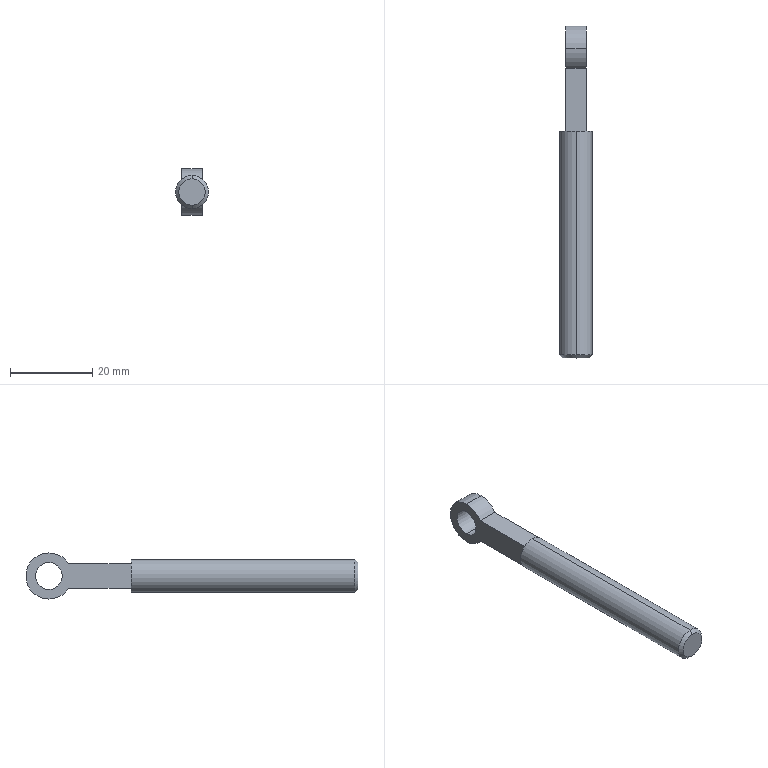Part | STEP file | tension screw_SUS304 | 1 solid | 15 faces | box 8 x 80.6 x 11.2 mm | volume 3524 mm3 | cylinder 7 | plane 6 | cone 2 | commonest cylinder face diameters 11.2 x3 6.5 x2 8 x2
STEP:
#1=CARTESIAN_POINT('',(0.,0.,0.));
#2=DIRECTION('',(0.,0.,1.));
#3=DIRECTION('',(1.,0.,0.));
#4=AXIS2_PLACEMENT_3D('',#1,#2,#3);
#5=CARTESIAN_POINT('',(2.5,-74.2,4.));
#6=VERTEX_POINT('',#5);
#7=CARTESIAN_POINT('',(2.5,-74.2,-4.));
#8=VERTEX_POINT('',#7);
#9=CARTESIAN_POINT('',(2.5,-74.2,0.));
#10=DIRECTION('',(0.,1.,0.));
#11=DIRECTION('',(0.,0.,1.));
#12=AXIS2_PLACEMENT_3D('',#9,#10,#11);
#13=CIRCLE('',#12,4.);
#14=CARTESIAN_POINT('',(2.5,-75.,0.));
#15=DIRECTION('',(0.,1.,0.));
#16=DIRECTION('',(0.,0.,1.));
#17=AXIS2_PLACEMENT_3D('',#14,#15,#16);
#18=CYLINDRICAL_SURFACE('',#17,4.);
#19=CARTESIAN_POINT('',(0.,0.8));
#20=DIRECTION('',(1.,0.));
#21=VECTOR('',#20,1.);
#22=LINE('',#19,#21);
#23=(GEOMETRIC_REPRESENTATION_CONTEXT(2)PARAMETRIC_REPRESENTATION_CONTEXT()REPRESENTATION_CONTEXT('',''));
#24=DEFINITIONAL_REPRESENTATION('',(#22),#23);
#25=PCURVE('',#18,#24);
#26=CARTESIAN_POINT('',(2.5,-74.2,0.));
#27=DIRECTION('',(0.,1.,0.));
#28=DIRECTION('',(0.,0.,1.));
#29=AXIS2_PLACEMENT_3D('',#26,#27,#28);
#30=CONICAL_SURFACE('',#29,4.,0.7854);
#31=CARTESIAN_POINT('',(0.,0.));
#32=DIRECTION('',(1.,0.));
#33=VECTOR('',#32,1.);
#34=LINE('',#31,#33);
#35=(GEOMETRIC_REPRESENTATION_CONTEXT(2)PARAMETRIC_REPRESENTATION_CONTEXT()REPRESENTATION_CONTEXT('',''));
#36=DEFINITIONAL_REPRESENTATION('',(#34),#35);
#37=PCURVE('',#30,#36);
#38=SURFACE_CURVE('',#13,(#25,#37),.PCURVE_S1.);
#39=EDGE_CURVE('',#6,#8,#38,.T.);
#40=ORIENTED_EDGE('',*,*,#39,.T.);
#41=CARTESIAN_POINT('',(2.5,-20.,-4.));
#42=VERTEX_POINT('',#41);
#43=CARTESIAN_POINT('',(2.5,-75.,-4.));
#44=DIRECTION('',(0.,1.,0.));
#45=VECTOR('',#44,1.);
#46=LINE('',#43,#45);
#47=CARTESIAN_POINT('',(3.142,0.));
#48=DIRECTION('',(0.,1.));
#49=VECTOR('',#48,1.);
#50=LINE('',#47,#49);
#51=(GEOMETRIC_REPRESENTATION_CONTEXT(2)PARAMETRIC_REPRESENTATION_CONTEXT()REPRESENTATION_CONTEXT('',''));
#52=DEFINITIONAL_REPRESENTATION('',(#50),#51);
#53=PCURVE('',#18,#52);
#54=CARTESIAN_POINT('',(2.5,-75.,0.));
#55=DIRECTION('',(0.,1.,0.));
#56=DIRECTION('',(0.,0.,1.));
#57=AXIS2_PLACEMENT_3D('',#54,#55,#56);
#58=CYLINDRICAL_SURFACE('',#57,4.);
#59=CARTESIAN_POINT('',(3.142,0.));
#60=DIRECTION('',(0.,1.));
#61=VECTOR('',#60,1.);
#62=LINE('',#59,#61);
#63=(GEOMETRIC_REPRESENTATION_CONTEXT(2)PARAMETRIC_REPRESENTATION_CONTEXT()REPRESENTATION_CONTEXT('',''));
#64=DEFINITIONAL_REPRESENTATION('',(#62),#63);
#65=PCURVE('',#58,#64);
#66=SURFACE_CURVE('',#46,(#53,#65),.PCURVE_S1.);
#67=EDGE_CURVE('',#8,#42,#66,.T.);
#68=ORIENTED_EDGE('',*,*,#67,.T.);
#69=CARTESIAN_POINT('',(2.5,-20.,4.));
#70=VERTEX_POINT('',#69);
#71=CARTESIAN_POINT('',(2.5,-20.,0.));
#72=DIRECTION('',(0.,-1.,0.));
#73=DIRECTION('',(0.,0.,1.));
#74=AXIS2_PLACEMENT_3D('',#71,#72,#73);
#75=CIRCLE('',#74,4.);
#76=CARTESIAN_POINT('',(6.283,55.));
#77=DIRECTION('',(-1.,0.));
#78=VECTOR('',#77,1.);
#79=LINE('',#76,#78);
#80=(GEOMETRIC_REPRESENTATION_CONTEXT(2)PARAMETRIC_REPRESENTATION_CONTEXT()REPRESENTATION_CONTEXT('',''));
#81=DEFINITIONAL_REPRESENTATION('',(#79),#80);
#82=PCURVE('',#18,#81);
#83=CARTESIAN_POINT('',(2.5,-20.,0.));
#84=DIRECTION('',(0.,-1.,0.));
#85=DIRECTION('',(0.,0.,-1.));
#86=AXIS2_PLACEMENT_3D('',#83,#84,#85);
#87=PLANE('',#86);
#88=CARTESIAN_POINT('',(0.,0.));
#89=DIRECTION('',(-1.,0.));
#90=AXIS2_PLACEMENT_2D('',#88,#89);
#91=CIRCLE('',#90,4.);
#92=(GEOMETRIC_REPRESENTATION_CONTEXT(2)PARAMETRIC_REPRESENTATION_CONTEXT()REPRESENTATION_CONTEXT('',''));
#93=DEFINITIONAL_REPRESENTATION('',(#91),#92);
#94=PCURVE('',#87,#93);
#95=SURFACE_CURVE('',#75,(#82,#94),.PCURVE_S1.);
#96=EDGE_CURVE('',#42,#70,#95,.T.);
#97=ORIENTED_EDGE('',*,*,#96,.T.);
#98=CARTESIAN_POINT('',(2.5,-75.,4.));
#99=DIRECTION('',(0.,1.,0.));
#100=VECTOR('',#99,1.);
#101=LINE('',#98,#100);
#102=CARTESIAN_POINT('',(0.,0.));
#103=DIRECTION('',(0.,1.));
#104=VECTOR('',#103,1.);
#105=LINE('',#102,#104);
#106=(GEOMETRIC_REPRESENTATION_CONTEXT(2)PARAMETRIC_REPRESENTATION_CONTEXT()REPRESENTATION_CONTEXT('',''));
#107=DEFINITIONAL_REPRESENTATION('',(#105),#106);
#108=PCURVE('',#18,#107);
#109=CARTESIAN_POINT('',(6.283,0.));
#110=DIRECTION('',(0.,1.));
#111=VECTOR('',#110,1.);
#112=LINE('',#109,#111);
#113=(GEOMETRIC_REPRESENTATION_CONTEXT(2)PARAMETRIC_REPRESENTATION_CONTEXT()REPRESENTATION_CONTEXT('',''));
#114=DEFINITIONAL_REPRESENTATION('',(#112),#113);
#115=PCURVE('',#58,#114);
#116=SURFACE_CURVE('',#101,(#108,#115),.PCURVE_S1.);
#117=EDGE_CURVE('',#6,#70,#116,.T.);
#118=ORIENTED_EDGE('',*,*,#117,.F.);
#119=EDGE_LOOP('',(#40,#68,#97,#118));
#120=FACE_BOUND('',#119,.T.);
#121=ADVANCED_FACE('',(#120),#18,.T.);
#122=CARTESIAN_POINT('',(2.5,-75.,3.2));
#123=VERTEX_POINT('',#122);
#124=CARTESIAN_POINT('',(2.5,-75.,-3.2));
#125=VERTEX_POINT('',#124);
#126=CARTESIAN_POINT('',(2.5,-75.,0.));
#127=DIRECTION('',(0.,1.,0.));
#128=DIRECTION('',(0.,0.,1.));
#129=AXIS2_PLACEMENT_3D('',#126,#127,#128);
#130=CIRCLE('',#129,3.2);
#131=CARTESIAN_POINT('',(0.,-0.8));
#132=DIRECTION('',(1.,0.));
#133=VECTOR('',#132,1.);
#134=LINE('',#131,#133);
#135=(GEOMETRIC_REPRESENTATION_CONTEXT(2)PARAMETRIC_REPRESENTATION_CONTEXT()REPRESENTATION_CONTEXT('',''));
#136=DEFINITIONAL_REPRESENTATION('',(#134),#135);
#137=PCURVE('',#30,#136);
#138=CARTESIAN_POINT('',(2.5,-75.,0.));
#139=DIRECTION('',(0.,-1.,0.));
#140=DIRECTION('',(0.,0.,-1.));
#141=AXIS2_PLACEMENT_3D('',#138,#139,#140);
#142=PLANE('',#141);
#143=CARTESIAN_POINT('',(-3.2,0.));
#144=CARTESIAN_POINT('',(-3.2,5.543));
#145=CARTESIAN_POINT('',(1.6,2.771));
#146=CARTESIAN_POINT('',(6.4,0.));
#147=CARTESIAN_POINT('',(1.6,-2.771));
#148=CARTESIAN_POINT('',(-3.2,-5.543));
#149=CARTESIAN_POINT('',(-3.2,0.));
#150=(BOUNDED_CURVE()B_SPLINE_CURVE(2,(#143,#144,#145,#146,#147,#148,#149),.UNSPECIFIED.,.T.,.F.)B_SPLINE_CURVE_WITH_KNOTS((1,2,2,2,2,1),(-2.094,0.,2.094,4.189,6.283,8.378),.UNSPECIFIED.)CURVE()GEOMETRIC_REPRESENTATION_ITEM()RATIONAL_B_SPLINE_CURVE((1.,0.5,1.,0.5,1.,0.5,1.))REPRESENTATION_ITEM(''));
#151=(GEOMETRIC_REPRESENTATION_CONTEXT(2)PARAMETRIC_REPRESENTATION_CONTEXT()REPRESENTATION_CONTEXT('',''));
#152=DEFINITIONAL_REPRESENTATION('',(#150),#151);
#153=PCURVE('',#142,#152);
#154=SURFACE_CURVE('',#130,(#137,#153),.PCURVE_S1.);
#155=EDGE_CURVE('',#123,#125,#154,.T.);
#156=ORIENTED_EDGE('',*,*,#155,.T.);
#157=CARTESIAN_POINT('',(2.5,-74.2,-4.));
#158=DIRECTION('',(0.,0.7071,-0.7071));
#159=VECTOR('',#158,1.);
#160=LINE('',#157,#159);
#161=CARTESIAN_POINT('',(3.142,0.));
#162=DIRECTION('',(0.,1.));
#163=VECTOR('',#162,1.);
#164=LINE('',#161,#163);
#165=(GEOMETRIC_REPRESENTATION_CONTEXT(2)PARAMETRIC_REPRESENTATION_CONTEXT()REPRESENTATION_CONTEXT('',''));
#166=DEFINITIONAL_REPRESENTATION('',(#164),#165);
#167=PCURVE('',#30,#166);
#168=CARTESIAN_POINT('',(2.5,-74.2,0.));
#169=DIRECTION('',(0.,1.,0.));
#170=DIRECTION('',(0.,0.,1.));
#171=AXIS2_PLACEMENT_3D('',#168,#169,#170);
#172=CONICAL_SURFACE('',#171,4.,0.7854);
#173=CARTESIAN_POINT('',(3.142,0.));
#174=DIRECTION('',(0.,1.));
#175=VECTOR('',#174,1.);
#176=LINE('',#173,#175);
#177=(GEOMETRIC_REPRESENTATION_CONTEXT(2)PARAMETRIC_REPRESENTATION_CONTEXT()REPRESENTATION_CONTEXT('',''));
#178=DEFINITIONAL_REPRESENTATION('',(#176),#177);
#179=PCURVE('',#172,#178);
#180=SURFACE_CURVE('',#160,(#167,#179),.PCURVE_S1.);
#181=EDGE_CURVE('',#125,#8,#180,.T.);
#182=ORIENTED_EDGE('',*,*,#181,.T.);
#183=ORIENTED_EDGE('',*,*,#39,.F.);
#184=CARTESIAN_POINT('',(2.5,-74.2,4.));
#185=DIRECTION('',(0.,0.7071,0.7071));
#186=VECTOR('',#185,1.);
#187=LINE('',#184,#186);
#188=CARTESIAN_POINT('',(0.,0.));
#189=DIRECTION('',(0.,1.));
#190=VECTOR('',#189,1.);
#191=LINE('',#188,#190);
#192=(GEOMETRIC_REPRESENTATION_CONTEXT(2)PARAMETRIC_REPRESENTATION_CONTEXT()REPRESENTATION_CONTEXT('',''));
#193=DEFINITIONAL_REPRESENTATION('',(#191),#192);
#194=PCURVE('',#30,#193);
#195=CARTESIAN_POINT('',(6.283,0.));
#196=DIRECTION('',(0.,1.));
#197=VECTOR('',#196,1.);
#198=LINE('',#195,#197);
#199=(GEOMETRIC_REPRESENTATION_CONTEXT(2)PARAMETRIC_REPRESENTATION_CONTEXT()REPRESENTATION_CONTEXT('',''));
#200=DEFINITIONAL_REPRESENTATION('',(#198),#199);
#201=PCURVE('',#172,#200);
#202=SURFACE_CURVE('',#187,(#194,#201),.PCURVE_S1.);
#203=EDGE_CURVE('',#123,#6,#202,.T.);
#204=ORIENTED_EDGE('',*,*,#203,.F.);
#205=EDGE_LOOP('',(#156,#182,#183,#204));
#206=FACE_BOUND('',#205,.T.);
#207=ADVANCED_FACE('',(#206),#30,.T.);
#208=CARTESIAN_POINT('',(5.,0.,-5.6));
#209=VERTEX_POINT('',#208);
#210=CARTESIAN_POINT('',(5.,0.,5.6));
#211=VERTEX_POINT('',#210);
#212=CARTESIAN_POINT('',(5.,0.,0.));
#213=DIRECTION('',(1.,0.,0.));
#214=DIRECTION('',(0.,0.,1.));
#215=AXIS2_PLACEMENT_3D('',#212,#213,#214);
#216=CIRCLE('',#215,5.6);
#217=CARTESIAN_POINT('',(5.,0.,0.));
#218=DIRECTION('',(-1.,0.,0.));
#219=DIRECTION('',(0.,0.,1.));
#220=AXIS2_PLACEMENT_3D('',#217,#218,#219);
#221=CYLINDRICAL_SURFACE('',#220,5.6);
#222=CARTESIAN_POINT('',(6.283,0.));
#223=DIRECTION('',(-1.,0.));
#224=VECTOR('',#223,1.);
#225=LINE('',#222,#224);
#226=(GEOMETRIC_REPRESENTATION_CONTEXT(2)PARAMETRIC_REPRESENTATION_CONTEXT()REPRESENTATION_CONTEXT('',''));
#227=DEFINITIONAL_REPRESENTATION('',(#225),#226);
#228=PCURVE('',#221,#227);
#229=CARTESIAN_POINT('',(5.,0.,0.));
#230=DIRECTION('',(1.,0.,0.));
#231=DIRECTION('',(0.,0.,-1.));
#232=AXIS2_PLACEMENT_3D('',#229,#230,#231);
#233=PLANE('',#232);
#234=CARTESIAN_POINT('',(0.,0.));
#235=DIRECTION('',(-1.,0.));
#236=AXIS2_PLACEMENT_2D('',#234,#235);
#237=CIRCLE('',#236,5.6);
#238=(GEOMETRIC_REPRESENTATION_CONTEXT(2)PARAMETRIC_REPRESENTATION_CONTEXT()REPRESENTATION_CONTEXT('',''));
#239=DEFINITIONAL_REPRESENTATION('',(#237),#238);
#240=PCURVE('',#233,#239);
#241=SURFACE_CURVE('',#216,(#228,#240),.PCURVE_S1.);
#242=EDGE_CURVE('',#209,#211,#241,.T.);
#243=ORIENTED_EDGE('',*,*,#242,.F.);
#244=CARTESIAN_POINT('',(0.,0.,-5.6));
#245=VERTEX_POINT('',#244);
#246=CARTESIAN_POINT('',(5.,0.,-5.6));
#247=DIRECTION('',(-1.,0.,0.));
#248=VECTOR('',#247,1.);
#249=LINE('',#246,#248);
#250=CARTESIAN_POINT('',(3.142,0.));
#251=DIRECTION('',(0.,1.));
#252=VECTOR('',#251,1.);
#253=LINE('',#250,#252);
#254=(GEOMETRIC_REPRESENTATION_CONTEXT(2)PARAMETRIC_REPRESENTATION_CONTEXT()REPRESENTATION_CONTEXT('',''));
#255=DEFINITIONAL_REPRESENTATION('',(#253),#254);
#256=PCURVE('',#221,#255);
#257=CARTESIAN_POINT('',(5.,0.,0.));
#258=DIRECTION('',(-1.,0.,0.));
#259=DIRECTION('',(0.,0.,1.));
#260=AXIS2_PLACEMENT_3D('',#257,#258,#259);
#261=CYLINDRICAL_SURFACE('',#260,5.6);
#262=CARTESIAN_POINT('',(3.142,0.));
#263=DIRECTION('',(0.,1.));
#264=VECTOR('',#263,1.);
#265=LINE('',#262,#264);
#266=(GEOMETRIC_REPRESENTATION_CONTEXT(2)PARAMETRIC_REPRESENTATION_CONTEXT()REPRESENTATION_CONTEXT('',''));
#267=DEFINITIONAL_REPRESENTATION('',(#265),#266);
#268=PCURVE('',#261,#267);
#269=SURFACE_CURVE('',#249,(#256,#268),.PCURVE_S1.);
#270=EDGE_CURVE('',#209,#245,#269,.T.);
#271=ORIENTED_EDGE('',*,*,#270,.T.);
#272=CARTESIAN_POINT('',(0.,0.,5.6));
#273=VERTEX_POINT('',#272);
#274=CARTESIAN_POINT('',(0.,0.,0.));
#275=DIRECTION('',(1.,0.,0.));
#276=DIRECTION('',(0.,0.,1.));
#277=AXIS2_PLACEMENT_3D('',#274,#275,#276);
#278=CIRCLE('',#277,5.6);
#279=CARTESIAN_POINT('',(6.283,5.));
#280=DIRECTION('',(-1.,0.));
#281=VECTOR('',#280,1.);
#282=LINE('',#279,#281);
#283=(GEOMETRIC_REPRESENTATION_CONTEXT(2)PARAMETRIC_REPRESENTATION_CONTEXT()REPRESENTATION_CONTEXT('',''));
#284=DEFINITIONAL_REPRESENTATION('',(#282),#283);
#285=PCURVE('',#221,#284);
#286=CARTESIAN_POINT('',(0.,0.,0.));
#287=DIRECTION('',(1.,0.,0.));
#288=DIRECTION('',(0.,0.,-1.));
#289=AXIS2_PLACEMENT_3D('',#286,#287,#288);
#290=PLANE('',#289);
#291=CARTESIAN_POINT('',(0.,0.));
#292=DIRECTION('',(-1.,0.));
#293=AXIS2_PLACEMENT_2D('',#291,#292);
#294=CIRCLE('',#293,5.6);
#295=(GEOMETRIC_REPRESENTATION_CONTEXT(2)PARAMETRIC_REPRESENTATION_CONTEXT()REPRESENTATION_CONTEXT('',''));
#296=DEFINITIONAL_REPRESENTATION('',(#294),#295);
#297=PCURVE('',#290,#296);
#298=SURFACE_CURVE('',#278,(#285,#297),.PCURVE_S1.);
#299=EDGE_CURVE('',#245,#273,#298,.T.);
#300=ORIENTED_EDGE('',*,*,#299,.T.);
#301=CARTESIAN_POINT('',(5.,0.,5.6));
#302=DIRECTION('',(-1.,0.,0.));
#303=VECTOR('',#302,1.);
#304=LINE('',#301,#303);
#305=CARTESIAN_POINT('',(0.,0.));
#306=DIRECTION('',(0.,1.));
#307=VECTOR('',#306,1.);
#308=LINE('',#305,#307);
#309=(GEOMETRIC_REPRESENTATION_CONTEXT(2)PARAMETRIC_REPRESENTATION_CONTEXT()REPRESENTATION_CONTEXT('',''));
#310=DEFINITIONAL_REPRESENTATION('',(#308),#309);
#311=PCURVE('',#221,#310);
#312=CARTESIAN_POINT('',(5.,0.,0.));
#313=DIRECTION('',(-1.,0.,0.));
#314=DIRECTION('',(0.,0.,1.));
#315=AXIS2_PLACEMENT_3D('',#312,#313,#314);
#316=CYLINDRICAL_SURFACE('',#315,5.6);
#317=CARTESIAN_POINT('',(6.283,0.));
#318=DIRECTION('',(0.,1.));
#319=VECTOR('',#318,1.);
#320=LINE('',#317,#319);
#321=(GEOMETRIC_REPRESENTATION_CONTEXT(2)PARAMETRIC_REPRESENTATION_CONTEXT()REPRESENTATION_CONTEXT('',''));
#322=DEFINITIONAL_REPRESENTATION('',(#320),#321);
#323=PCURVE('',#316,#322);
#324=SURFACE_CURVE('',#304,(#311,#323),.PCURVE_S1.);
#325=EDGE_CURVE('',#211,#273,#324,.T.);
#326=ORIENTED_EDGE('',*,*,#325,.F.);
#327=EDGE_LOOP('',(#243,#271,#300,#326));
#328=FACE_BOUND('',#327,.T.);
#329=ADVANCED_FACE('',(#328),#221,.T.);
#330=CARTESIAN_POINT('',(5.,-4.729,3.));
#331=VERTEX_POINT('',#330);
#332=CARTESIAN_POINT('',(5.,0.,0.));
#333=DIRECTION('',(1.,0.,0.));
#334=DIRECTION('',(0.,0.,1.));
#335=AXIS2_PLACEMENT_3D('',#332,#333,#334);
#336=CIRCLE('',#335,5.6);
#337=CARTESIAN_POINT('',(6.283,0.));
#338=DIRECTION('',(-1.,0.));
#339=VECTOR('',#338,1.);
#340=LINE('',#337,#339);
#341=(GEOMETRIC_REPRESENTATION_CONTEXT(2)PARAMETRIC_REPRESENTATION_CONTEXT()REPRESENTATION_CONTEXT('',''));
#342=DEFINITIONAL_REPRESENTATION('',(#340),#341);
#343=PCURVE('',#316,#342);
#344=CARTESIAN_POINT('',(0.,0.));
#345=DIRECTION('',(-1.,0.));
#346=AXIS2_PLACEMENT_2D('',#344,#345);
#347=CIRCLE('',#346,5.6);
#348=(GEOMETRIC_REPRESENTATION_CONTEXT(2)PARAMETRIC_REPRESENTATION_CONTEXT()REPRESENTATION_CONTEXT('',''));
#349=DEFINITIONAL_REPRESENTATION('',(#347),#348);
#350=PCURVE('',#233,#349);
#351=SURFACE_CURVE('',#336,(#343,#350),.PCURVE_S1.);
#352=EDGE_CURVE('',#211,#331,#351,.T.);
#353=ORIENTED_EDGE('',*,*,#352,.F.);
#354=ORIENTED_EDGE('',*,*,#325,.T.);
#355=CARTESIAN_POINT('',(0.,-4.729,3.));
#356=VERTEX_POINT('',#355);
#357=CARTESIAN_POINT('',(0.,0.,0.));
#358=DIRECTION('',(1.,0.,0.));
#359=DIRECTION('',(0.,0.,1.));
#360=AXIS2_PLACEMENT_3D('',#357,#358,#359);
#361=CIRCLE('',#360,5.6);
#362=CARTESIAN_POINT('',(6.283,5.));
#363=DIRECTION('',(-1.,0.));
#364=VECTOR('',#363,1.);
#365=LINE('',#362,#364);
#366=(GEOMETRIC_REPRESENTATION_CONTEXT(2)PARAMETRIC_REPRESENTATION_CONTEXT()REPRESENTATION_CONTEXT('',''));
#367=DEFINITIONAL_REPRESENTATION('',(#365),#366);
#368=PCURVE('',#316,#367);
#369=CARTESIAN_POINT('',(0.,0.));
#370=DIRECTION('',(-1.,0.));
#371=AXIS2_PLACEMENT_2D('',#369,#370);
#372=CIRCLE('',#371,5.6);
#373=(GEOMETRIC_REPRESENTATION_CONTEXT(2)PARAMETRIC_REPRESENTATION_CONTEXT()REPRESENTATION_CONTEXT('',''));
#374=DEFINITIONAL_REPRESENTATION('',(#372),#373);
#375=PCURVE('',#290,#374);
#376=SURFACE_CURVE('',#361,(#368,#375),.PCURVE_S1.);
#377=EDGE_CURVE('',#273,#356,#376,.T.);
#378=ORIENTED_EDGE('',*,*,#377,.T.);
#379=CARTESIAN_POINT('',(5.,-4.729,3.));
#380=DIRECTION('',(1.,0.,0.));
#381=VECTOR('',#380,1.);
#382=LINE('',#379,#381);
#383=CARTESIAN_POINT('',(5.278,0.));
#384=DIRECTION('',(0.,-1.));
#385=VECTOR('',#384,1.);
#386=LINE('',#383,#385);
#387=(GEOMETRIC_REPRESENTATION_CONTEXT(2)PARAMETRIC_REPRESENTATION_CONTEXT()REPRESENTATION_CONTEXT('',''));
#388=DEFINITIONAL_REPRESENTATION('',(#386),#387);
#389=PCURVE('',#316,#388);
#390=CARTESIAN_POINT('',(5.,-4.729,3.));
#391=DIRECTION('',(0.,0.,-1.));
#392=DIRECTION('',(0.,1.,0.));
#393=AXIS2_PLACEMENT_3D('',#390,#391,#392);
#394=PLANE('',#393);
#395=CARTESIAN_POINT('',(0.,0.));
#396=DIRECTION('',(0.,1.));
#397=VECTOR('',#396,1.);
#398=LINE('',#395,#397);
#399=(GEOMETRIC_REPRESENTATION_CONTEXT(2)PARAMETRIC_REPRESENTATION_CONTEXT()REPRESENTATION_CONTEXT('',''));
#400=DEFINITIONAL_REPRESENTATION('',(#398),#399);
#401=PCURVE('',#394,#400);
#402=SURFACE_CURVE('',#382,(#389,#401),.PCURVE_S1.);
#403=EDGE_CURVE('',#356,#331,#402,.T.);
#404=ORIENTED_EDGE('',*,*,#403,.T.);
#405=EDGE_LOOP('',(#353,#354,#378,#404));
#406=FACE_BOUND('',#405,.T.);
#407=ADVANCED_FACE('',(#406),#316,.T.);
#408=CARTESIAN_POINT('',(5.,0.,3.25));
#409=VERTEX_POINT('',#408);
#410=CARTESIAN_POINT('',(0.,0.,3.25));
#411=VERTEX_POINT('',#410);
#412=CARTESIAN_POINT('',(5.,0.,3.25));
#413=DIRECTION('',(-1.,0.,0.));
#414=VECTOR('',#413,1.);
#415=LINE('',#412,#414);
#416=CARTESIAN_POINT('',(5.,0.,0.));
#417=DIRECTION('',(-1.,0.,0.));
#418=DIRECTION('',(0.,0.,1.));
#419=AXIS2_PLACEMENT_3D('',#416,#417,#418);
#420=CYLINDRICAL_SURFACE('',#419,3.25);
#421=CARTESIAN_POINT('',(6.283,0.));
#422=DIRECTION('',(0.,1.));
#423=VECTOR('',#422,1.);
#424=LINE('',#421,#423);
#425=(GEOMETRIC_REPRESENTATION_CONTEXT(2)PARAMETRIC_REPRESENTATION_CONTEXT()REPRESENTATION_CONTEXT('',''));
#426=DEFINITIONAL_REPRESENTATION('',(#424),#425);
#427=PCURVE('',#420,#426);
#428=CARTESIAN_POINT('',(5.,0.,0.));
#429=DIRECTION('',(-1.,0.,0.));
#430=DIRECTION('',(0.,0.,1.));
#431=AXIS2_PLACEMENT_3D('',#428,#429,#430);
#432=CYLINDRICAL_SURFACE('',#431,3.25);
#433=CARTESIAN_POINT('',(0.,0.));
#434=DIRECTION('',(0.,1.));
#435=VECTOR('',#434,1.);
#436=LINE('',#433,#435);
#437=(GEOMETRIC_REPRESENTATION_CONTEXT(2)PARAMETRIC_REPRESENTATION_CONTEXT()REPRESENTATION_CONTEXT('',''));
#438=DEFINITIONAL_REPRESENTATION('',(#436),#437);
#439=PCURVE('',#432,#438);
#440=SURFACE_CURVE('',#415,(#427,#439),.PCURVE_S1.);
#441=EDGE_CURVE('',#409,#411,#440,.T.);
#442=ORIENTED_EDGE('',*,*,#441,.T.);
#443=CARTESIAN_POINT('',(0.,0.,-3.25));
#444=VERTEX_POINT('',#443);
#445=CARTESIAN_POINT('',(0.,0.,0.));
#446=DIRECTION('',(-1.,0.,0.));
#447=DIRECTION('',(0.,0.,1.));
#448=AXIS2_PLACEMENT_3D('',#445,#446,#447);
#449=CIRCLE('',#448,3.25);
#450=CARTESIAN_POINT('',(0.,5.));
#451=DIRECTION('',(1.,0.));
#452=VECTOR('',#451,1.);
#453=LINE('',#450,#452);
#454=(GEOMETRIC_REPRESENTATION_CONTEXT(2)PARAMETRIC_REPRESENTATION_CONTEXT()REPRESENTATION_CONTEXT('',''));
#455=DEFINITIONAL_REPRESENTATION('',(#453),#454);
#456=PCURVE('',#420,#455);
#457=CARTESIAN_POINT('',(-3.25,0.));
#458=CARTESIAN_POINT('',(-3.25,5.629));
#459=CARTESIAN_POINT('',(1.625,2.815));
#460=CARTESIAN_POINT('',(6.5,0.));
#461=CARTESIAN_POINT('',(1.625,-2.815));
#462=CARTESIAN_POINT('',(-3.25,-5.629));
#463=CARTESIAN_POINT('',(-3.25,0.));
#464=(BOUNDED_CURVE()B_SPLINE_CURVE(2,(#457,#458,#459,#460,#461,#462,#463),.UNSPECIFIED.,.T.,.F.)B_SPLINE_CURVE_WITH_KNOTS((1,2,2,2,2,1),(-2.094,0.,2.094,4.189,6.283,8.378),.UNSPECIFIED.)CURVE()GEOMETRIC_REPRESENTATION_ITEM()RATIONAL_B_SPLINE_CURVE((1.,0.5,1.,0.5,1.,0.5,1.))REPRESENTATION_ITEM(''));
#465=(GEOMETRIC_REPRESENTATION_CONTEXT(2)PARAMETRIC_REPRESENTATION_CONTEXT()REPRESENTATION_CONTEXT('',''));
#466=DEFINITIONAL_REPRESENTATION('',(#464),#465);
#467=PCURVE('',#290,#466);
#468=SURFACE_CURVE('',#449,(#456,#467),.PCURVE_S1.);
#469=EDGE_CURVE('',#444,#411,#468,.T.);
#470=ORIENTED_EDGE('',*,*,#469,.F.);
#471=CARTESIAN_POINT('',(5.,0.,-3.25));
#472=VERTEX_POINT('',#471);
#473=CARTESIAN_POINT('',(5.,0.,-3.25));
#474=DIRECTION('',(-1.,0.,0.));
#475=VECTOR('',#474,1.);
#476=LINE('',#473,#475);
#477=CARTESIAN_POINT('',(3.142,0.));
#478=DIRECTION('',(0.,1.));
#479=VECTOR('',#478,1.);
#480=LINE('',#477,#479);
#481=(GEOMETRIC_REPRESENTATION_CONTEXT(2)PARAMETRIC_REPRESENTATION_CONTEXT()REPRESENTATION_CONTEXT('',''));
#482=DEFINITIONAL_REPRESENTATION('',(#480),#481);
#483=PCURVE('',#420,#482);
#484=CARTESIAN_POINT('',(3.142,0.));
#485=DIRECTION('',(0.,1.));
#486=VECTOR('',#485,1.);
#487=LINE('',#484,#486);
#488=(GEOMETRIC_REPRESENTATION_CONTEXT(2)PARAMETRIC_REPRESENTATION_CONTEXT()REPRESENTATION_CONTEXT('',''));
#489=DEFINITIONAL_REPRESENTATION('',(#487),#488);
#490=PCURVE('',#432,#489);
#491=SURFACE_CURVE('',#476,(#483,#490),.PCURVE_S1.);
#492=EDGE_CURVE('',#472,#444,#491,.T.);
#493=ORIENTED_EDGE('',*,*,#492,.F.);
#494=CARTESIAN_POINT('',(5.,0.,0.));
#495=DIRECTION('',(-1.,0.,0.));
#496=DIRECTION('',(0.,0.,1.));
#497=AXIS2_PLACEMENT_3D('',#494,#495,#496);
#498=CIRCLE('',#497,3.25);
#499=CARTESIAN_POINT('',(0.,0.));
#500=DIRECTION('',(1.,0.));
#501=VECTOR('',#500,1.);
#502=LINE('',#499,#501);
#503=(GEOMETRIC_REPRESENTATION_CONTEXT(2)PARAMETRIC_REPRESENTATION_CONTEXT()REPRESENTATION_CONTEXT('',''));
#504=DEFINITIONAL_REPRESENTATION('',(#502),#503);
#505=PCURVE('',#420,#504);
#506=CARTESIAN_POINT('',(-3.25,0.));
#507=CARTESIAN_POINT('',(-3.25,5.629));
#508=CARTESIAN_POINT('',(1.625,2.815));
#509=CARTESIAN_POINT('',(6.5,0.));
#510=CARTESIAN_POINT('',(1.625,-2.815));
#511=CARTESIAN_POINT('',(-3.25,-5.629));
#512=CARTESIAN_POINT('',(-3.25,0.));
#513=(BOUNDED_CURVE()B_SPLINE_CURVE(2,(#506,#507,#508,#509,#510,#511,#512),.UNSPECIFIED.,.T.,.F.)B_SPLINE_CURVE_WITH_KNOTS((1,2,2,2,2,1),(-2.094,0.,2.094,4.189,6.283,8.378),.UNSPECIFIED.)CURVE()GEOMETRIC_REPRESENTATION_ITEM()RATIONAL_B_SPLINE_CURVE((1.,0.5,1.,0.5,1.,0.5,1.))REPRESENTATION_ITEM(''));
#514=(GEOMETRIC_REPRESENTATION_CONTEXT(2)PARAMETRIC_REPRESENTATION_CONTEXT()REPRESENTATION_CONTEXT('',''));
#515=DEFINITIONAL_REPRESENTATION('',(#513),#514);
#516=PCURVE('',#233,#515);
#517=SURFACE_CURVE('',#498,(#505,#516),.PCURVE_S1.);
#518=EDGE_CURVE('',#472,#409,#517,.T.);
#519=ORIENTED_EDGE('',*,*,#518,.T.);
#520=EDGE_LOOP('',(#442,#470,#493,#519));
#521=FACE_BOUND('',#520,.F.);
#522=ADVANCED_FACE('',(#521),#420,.F.);
#523=ORIENTED_EDGE('',*,*,#67,.F.);
#524=CARTESIAN_POINT('',(2.5,-74.2,0.));
#525=DIRECTION('',(0.,1.,0.));
#526=DIRECTION('',(0.,0.,1.));
#527=AXIS2_PLACEMENT_3D('',#524,#525,#526);
#528=CIRCLE('',#527,4.);
#529=CARTESIAN_POINT('',(0.,0.8));
#530=DIRECTION('',(1.,0.));
#531=VECTOR('',#530,1.);
#532=LINE('',#529,#531);
#533=(GEOMETRIC_REPRESENTATION_CONTEXT(2)PARAMETRIC_REPRESENTATION_CONTEXT()REPRESENTATION_CONTEXT('',''));
#534=DEFINITIONAL_REPRESENTATION('',(#532),#533);
#535=PCURVE('',#58,#534);
#536=CARTESIAN_POINT('',(0.,0.));
#537=DIRECTION('',(1.,0.));
#538=VECTOR('',#537,1.);
#539=LINE('',#536,#538);
#540=(GEOMETRIC_REPRESENTATION_CONTEXT(2)PARAMETRIC_REPRESENTATION_CONTEXT()REPRESENTATION_CONTEXT('',''));
#541=DEFINITIONAL_REPRESENTATION('',(#539),#540);
#542=PCURVE('',#172,#541);
#543=SURFACE_CURVE('',#528,(#535,#542),.PCURVE_S1.);
#544=EDGE_CURVE('',#8,#6,#543,.T.);
#545=ORIENTED_EDGE('',*,*,#544,.T.);
#546=ORIENTED_EDGE('',*,*,#117,.T.);
#547=CARTESIAN_POINT('',(2.5,-20.,0.));
#548=DIRECTION('',(0.,-1.,0.));
#549=DIRECTION('',(0.,0.,1.));
#550=AXIS2_PLACEMENT_3D('',#547,#548,#549);
#551=CIRCLE('',#550,4.);
#552=CARTESIAN_POINT('',(6.283,55.));
#553=DIRECTION('',(-1.,0.));
#554=VECTOR('',#553,1.);
#555=LINE('',#552,#554);
#556=(GEOMETRIC_REPRESENTATION_CONTEXT(2)PARAMETRIC_REPRESENTATION_CONTEXT()REPRESENTATION_CONTEXT('',''));
#557=DEFINITIONAL_REPRESENTATION('',(#555),#556);
#558=PCURVE('',#58,#557);
#559=CARTESIAN_POINT('',(0.,0.));
#560=DIRECTION('',(-1.,0.));
#561=AXIS2_PLACEMENT_2D('',#559,#560);
#562=CIRCLE('',#561,4.);
#563=(GEOMETRIC_REPRESENTATION_CONTEXT(2)PARAMETRIC_REPRESENTATION_CONTEXT()REPRESENTATION_CONTEXT('',''));
#564=DEFINITIONAL_REPRESENTATION('',(#562),#563);
#565=PCURVE('',#87,#564);
#566=SURFACE_CURVE('',#551,(#558,#565),.PCURVE_S1.);
#567=EDGE_CURVE('',#70,#42,#566,.T.);
#568=ORIENTED_EDGE('',*,*,#567,.T.);
#569=EDGE_LOOP('',(#523,#545,#546,#568));
#570=FACE_BOUND('',#569,.T.);
#571=ADVANCED_FACE('',(#570),#58,.T.);
#572=ORIENTED_EDGE('',*,*,#567,.F.);
#573=ORIENTED_EDGE('',*,*,#96,.F.);
#574=EDGE_LOOP('',(#572,#573));
#575=FACE_BOUND('',#574,.T.);
#576=CARTESIAN_POINT('',(5.,-20.,3.));
#577=VERTEX_POINT('',#576);
#578=CARTESIAN_POINT('',(5.,-20.,-3.));
#579=VERTEX_POINT('',#578);
#580=CARTESIAN_POINT('',(5.,-20.,0.));
#581=DIRECTION('',(0.,0.,-1.));
#582=VECTOR('',#581,1.);
#583=LINE('',#580,#582);
#584=CARTESIAN_POINT('',(0.,2.5));
#585=DIRECTION('',(1.,0.));
#586=VECTOR('',#585,1.);
#587=LINE('',#584,#586);
#588=(GEOMETRIC_REPRESENTATION_CONTEXT(2)PARAMETRIC_REPRESENTATION_CONTEXT()REPRESENTATION_CONTEXT('',''));
#589=DEFINITIONAL_REPRESENTATION('',(#587),#588);
#590=PCURVE('',#87,#589);
#591=CARTESIAN_POINT('',(0.,-20.));
#592=DIRECTION('',(1.,0.));
#593=VECTOR('',#592,1.);
#594=LINE('',#591,#593);
#595=(GEOMETRIC_REPRESENTATION_CONTEXT(2)PARAMETRIC_REPRESENTATION_CONTEXT()REPRESENTATION_CONTEXT('',''));
#596=DEFINITIONAL_REPRESENTATION('',(#594),#595);
#597=PCURVE('',#233,#596);
#598=SURFACE_CURVE('',#583,(#590,#597),.PCURVE_S1.);
#599=EDGE_CURVE('',#577,#579,#598,.T.);
#600=ORIENTED_EDGE('',*,*,#599,.F.);
#601=CARTESIAN_POINT('',(0.,-20.,3.));
#602=VERTEX_POINT('',#601);
#603=CARTESIAN_POINT('',(2.5,-20.,3.));
#604=DIRECTION('',(1.,0.,0.));
#605=VECTOR('',#604,1.);
#606=LINE('',#603,#605);
#607=CARTESIAN_POINT('',(-3.,0.));
#608=DIRECTION('',(0.,1.));
#609=VECTOR('',#608,1.);
#610=LINE('',#607,#609);
#611=(GEOMETRIC_REPRESENTATION_CONTEXT(2)PARAMETRIC_REPRESENTATION_CONTEXT()REPRESENTATION_CONTEXT('',''));
#612=DEFINITIONAL_REPRESENTATION('',(#610),#611);
#613=PCURVE('',#87,#612);
#614=CARTESIAN_POINT('',(-15.271,-2.5));
#615=DIRECTION('',(0.,1.));
#616=VECTOR('',#615,1.);
#617=LINE('',#614,#616);
#618=(GEOMETRIC_REPRESENTATION_CONTEXT(2)PARAMETRIC_REPRESENTATION_CONTEXT()REPRESENTATION_CONTEXT('',''));
#619=DEFINITIONAL_REPRESENTATION('',(#617),#618);
#620=PCURVE('',#394,#619);
#621=SURFACE_CURVE('',#606,(#613,#620),.PCURVE_S1.);
#622=EDGE_CURVE('',#602,#577,#621,.T.);
#623=ORIENTED_EDGE('',*,*,#622,.F.);
#624=CARTESIAN_POINT('',(0.,-20.,-3.));
#625=VERTEX_POINT('',#624);
#626=CARTESIAN_POINT('',(0.,-20.,0.));
#627=DIRECTION('',(0.,0.,1.));
#628=VECTOR('',#627,1.);
#629=LINE('',#626,#628);
#630=CARTESIAN_POINT('',(0.,-2.5));
#631=DIRECTION('',(-1.,0.));
#632=VECTOR('',#631,1.);
#633=LINE('',#630,#632);
#634=(GEOMETRIC_REPRESENTATION_CONTEXT(2)PARAMETRIC_REPRESENTATION_CONTEXT()REPRESENTATION_CONTEXT('',''));
#635=DEFINITIONAL_REPRESENTATION('',(#633),#634);
#636=PCURVE('',#87,#635);
#637=CARTESIAN_POINT('',(0.,-20.));
#638=DIRECTION('',(-1.,0.));
#639=VECTOR('',#638,1.);
#640=LINE('',#637,#639);
#641=(GEOMETRIC_REPRESENTATION_CONTEXT(2)PARAMETRIC_REPRESENTATION_CONTEXT()REPRESENTATION_CONTEXT('',''));
#642=DEFINITIONAL_REPRESENTATION('',(#640),#641);
#643=PCURVE('',#290,#642);
#644=SURFACE_CURVE('',#629,(#636,#643),.PCURVE_S1.);
#645=EDGE_CURVE('',#625,#602,#644,.T.);
#646=ORIENTED_EDGE('',*,*,#645,.F.);
#647=CARTESIAN_POINT('',(2.5,-20.,-3.));
#648=DIRECTION('',(-1.,0.,0.));
#649=VECTOR('',#648,1.);
#650=LINE('',#647,#649);
#651=CARTESIAN_POINT('',(3.,0.));
#652=DIRECTION('',(0.,-1.));
#653=VECTOR('',#652,1.);
#654=LINE('',#651,#653);
#655=(GEOMETRIC_REPRESENTATION_CONTEXT(2)PARAMETRIC_REPRESENTATION_CONTEXT()REPRESENTATION_CONTEXT('',''));
#656=DEFINITIONAL_REPRESENTATION('',(#654),#655);
#657=PCURVE('',#87,#656);
#658=CARTESIAN_POINT('',(5.,-4.729,-3.));
#659=DIRECTION('',(0.,0.,1.));
#660=DIRECTION('',(0.,-1.,0.));
#661=AXIS2_PLACEMENT_3D('',#658,#659,#660);
#662=PLANE('',#661);
#663=CARTESIAN_POINT('',(15.271,-2.5));
#664=DIRECTION('',(0.,-1.));
#665=VECTOR('',#664,1.);
#666=LINE('',#663,#665);
#667=(GEOMETRIC_REPRESENTATION_CONTEXT(2)PARAMETRIC_REPRESENTATION_CONTEXT()REPRESENTATION_CONTEXT('',''));
#668=DEFINITIONAL_REPRESENTATION('',(#666),#667);
#669=PCURVE('',#662,#668);
#670=SURFACE_CURVE('',#650,(#657,#669),.PCURVE_S1.);
#671=EDGE_CURVE('',#579,#625,#670,.T.);
#672=ORIENTED_EDGE('',*,*,#671,.F.);
#673=EDGE_LOOP('',(#600,#623,#646,#672));
#674=FACE_BOUND('',#673,.T.);
#675=ADVANCED_FACE('',(#575,#674),#87,.F.);
#676=ORIENTED_EDGE('',*,*,#181,.F.);
#677=CARTESIAN_POINT('',(2.5,-75.,0.));
#678=DIRECTION('',(0.,1.,0.));
#679=DIRECTION('',(0.,0.,1.));
#680=AXIS2_PLACEMENT_3D('',#677,#678,#679);
#681=CIRCLE('',#680,3.2);
#682=CARTESIAN_POINT('',(0.,-0.8));
#683=DIRECTION('',(1.,0.));
#684=VECTOR('',#683,1.);
#685=LINE('',#682,#684);
#686=(GEOMETRIC_REPRESENTATION_CONTEXT(2)PARAMETRIC_REPRESENTATION_CONTEXT()REPRESENTATION_CONTEXT('',''));
#687=DEFINITIONAL_REPRESENTATION('',(#685),#686);
#688=PCURVE('',#172,#687);
#689=CARTESIAN_POINT('',(-3.2,0.));
#690=CARTESIAN_POINT('',(-3.2,5.543));
#691=CARTESIAN_POINT('',(1.6,2.771));
#692=CARTESIAN_POINT('',(6.4,0.));
#693=CARTESIAN_POINT('',(1.6,-2.771));
#694=CARTESIAN_POINT('',(-3.2,-5.543));
#695=CARTESIAN_POINT('',(-3.2,0.));
#696=(BOUNDED_CURVE()B_SPLINE_CURVE(2,(#689,#690,#691,#692,#693,#694,#695),.UNSPECIFIED.,.T.,.F.)B_SPLINE_CURVE_WITH_KNOTS((1,2,2,2,2,1),(-2.094,0.,2.094,4.189,6.283,8.378),.UNSPECIFIED.)CURVE()GEOMETRIC_REPRESENTATION_ITEM()RATIONAL_B_SPLINE_CURVE((1.,0.5,1.,0.5,1.,0.5,1.))REPRESENTATION_ITEM(''));
#697=(GEOMETRIC_REPRESENTATION_CONTEXT(2)PARAMETRIC_REPRESENTATION_CONTEXT()REPRESENTATION_CONTEXT('',''));
#698=DEFINITIONAL_REPRESENTATION('',(#696),#697);
#699=PCURVE('',#142,#698);
#700=SURFACE_CURVE('',#681,(#688,#699),.PCURVE_S1.);
#701=EDGE_CURVE('',#125,#123,#700,.T.);
#702=ORIENTED_EDGE('',*,*,#701,.T.);
#703=ORIENTED_EDGE('',*,*,#203,.T.);
#704=ORIENTED_EDGE('',*,*,#544,.F.);
#705=EDGE_LOOP('',(#676,#702,#703,#704));
#706=FACE_BOUND('',#705,.T.);
#707=ADVANCED_FACE('',(#706),#172,.T.);
#708=CARTESIAN_POINT('',(5.,-4.729,-3.));
#709=VERTEX_POINT('',#708);
#710=CARTESIAN_POINT('',(5.,-4.729,-3.));
#711=DIRECTION('',(0.,1.,0.));
#712=VECTOR('',#711,1.);
#713=LINE('',#710,#712);
#714=CARTESIAN_POINT('',(0.,0.));
#715=DIRECTION('',(-1.,0.));
#716=VECTOR('',#715,1.);
#717=LINE('',#714,#716);
#718=(GEOMETRIC_REPRESENTATION_CONTEXT(2)PARAMETRIC_REPRESENTATION_CONTEXT()REPRESENTATION_CONTEXT('',''));
#719=DEFINITIONAL_REPRESENTATION('',(#717),#718);
#720=PCURVE('',#662,#719);
#721=CARTESIAN_POINT('',(3.,-4.729));
#722=DIRECTION('',(0.,1.));
#723=VECTOR('',#722,1.);
#724=LINE('',#721,#723);
#725=(GEOMETRIC_REPRESENTATION_CONTEXT(2)PARAMETRIC_REPRESENTATION_CONTEXT()REPRESENTATION_CONTEXT('',''));
#726=DEFINITIONAL_REPRESENTATION('',(#724),#725);
#727=PCURVE('',#233,#726);
#728=SURFACE_CURVE('',#713,(#720,#727),.PCURVE_S1.);
#729=EDGE_CURVE('',#579,#709,#728,.T.);
#730=ORIENTED_EDGE('',*,*,#729,.F.);
#731=ORIENTED_EDGE('',*,*,#671,.T.);
#732=CARTESIAN_POINT('',(0.,-4.729,-3.));
#733=VERTEX_POINT('',#732);
#734=CARTESIAN_POINT('',(0.,-4.729,-3.));
#735=DIRECTION('',(0.,-1.,0.));
#736=VECTOR('',#735,1.);
#737=LINE('',#734,#736);
#738=CARTESIAN_POINT('',(0.,-5.));
#739=DIRECTION('',(1.,0.));
#740=VECTOR('',#739,1.);
#741=LINE('',#738,#740);
#742=(GEOMETRIC_REPRESENTATION_CONTEXT(2)PARAMETRIC_REPRESENTATION_CONTEXT()REPRESENTATION_CONTEXT('',''));
#743=DEFINITIONAL_REPRESENTATION('',(#741),#742);
#744=PCURVE('',#662,#743);
#745=CARTESIAN_POINT('',(3.,-4.729));
#746=DIRECTION('',(0.,-1.));
#747=VECTOR('',#746,1.);
#748=LINE('',#745,#747);
#749=(GEOMETRIC_REPRESENTATION_CONTEXT(2)PARAMETRIC_REPRESENTATION_CONTEXT()REPRESENTATION_CONTEXT('',''));
#750=DEFINITIONAL_REPRESENTATION('',(#748),#749);
#751=PCURVE('',#290,#750);
#752=SURFACE_CURVE('',#737,(#744,#751),.PCURVE_S1.);
#753=EDGE_CURVE('',#733,#625,#752,.T.);
#754=ORIENTED_EDGE('',*,*,#753,.F.);
#755=CARTESIAN_POINT('',(5.,-4.729,-3.));
#756=DIRECTION('',(-1.,0.,0.));
#757=VECTOR('',#756,1.);
#758=LINE('',#755,#757);
#759=CARTESIAN_POINT('',(0.,0.));
#760=DIRECTION('',(0.,-1.));
#761=VECTOR('',#760,1.);
#762=LINE('',#759,#761);
#763=(GEOMETRIC_REPRESENTATION_CONTEXT(2)PARAMETRIC_REPRESENTATION_CONTEXT()REPRESENTATION_CONTEXT('',''));
#764=DEFINITIONAL_REPRESENTATION('',(#762),#763);
#765=PCURVE('',#662,#764);
#766=CARTESIAN_POINT('',(4.147,0.));
#767=DIRECTION('',(0.,1.));
#768=VECTOR('',#767,1.);
#769=LINE('',#766,#768);
#770=(GEOMETRIC_REPRESENTATION_CONTEXT(2)PARAMETRIC_REPRESENTATION_CONTEXT()REPRESENTATION_CONTEXT('',''));
#771=DEFINITIONAL_REPRESENTATION('',(#769),#770);
#772=PCURVE('',#261,#771);
#773=SURFACE_CURVE('',#758,(#765,#772),.PCURVE_S1.);
#774=EDGE_CURVE('',#709,#733,#773,.T.);
#775=ORIENTED_EDGE('',*,*,#774,.F.);
#776=EDGE_LOOP('',(#730,#731,#754,#775));
#777=FACE_BOUND('',#776,.T.);
#778=ADVANCED_FACE('',(#777),#662,.F.);
#779=ORIENTED_EDGE('',*,*,#729,.T.);
#780=CARTESIAN_POINT('',(5.,0.,0.));
#781=DIRECTION('',(1.,0.,0.));
#782=DIRECTION('',(0.,0.,1.));
#783=AXIS2_PLACEMENT_3D('',#780,#781,#782);
#784=CIRCLE('',#783,5.6);
#785=CARTESIAN_POINT('',(0.,0.));
#786=DIRECTION('',(-1.,0.));
#787=AXIS2_PLACEMENT_2D('',#785,#786);
#788=CIRCLE('',#787,5.6);
#789=(GEOMETRIC_REPRESENTATION_CONTEXT(2)PARAMETRIC_REPRESENTATION_CONTEXT()REPRESENTATION_CONTEXT('',''));
#790=DEFINITIONAL_REPRESENTATION('',(#788),#789);
#791=PCURVE('',#233,#790);
#792=CARTESIAN_POINT('',(6.283,0.));
#793=DIRECTION('',(-1.,0.));
#794=VECTOR('',#793,1.);
#795=LINE('',#792,#794);
#796=(GEOMETRIC_REPRESENTATION_CONTEXT(2)PARAMETRIC_REPRESENTATION_CONTEXT()REPRESENTATION_CONTEXT('',''));
#797=DEFINITIONAL_REPRESENTATION('',(#795),#796);
#798=PCURVE('',#261,#797);
#799=SURFACE_CURVE('',#784,(#791,#798),.PCURVE_S1.);
#800=EDGE_CURVE('',#709,#209,#799,.T.);
#801=ORIENTED_EDGE('',*,*,#800,.T.);
#802=ORIENTED_EDGE('',*,*,#242,.T.);
#803=ORIENTED_EDGE('',*,*,#352,.T.);
#804=CARTESIAN_POINT('',(5.,0.,3.));
#805=DIRECTION('',(0.,-1.,0.));
#806=VECTOR('',#805,1.);
#807=LINE('',#804,#806);
#808=CARTESIAN_POINT('',(-3.,0.));
#809=DIRECTION('',(0.,-1.));
#810=VECTOR('',#809,1.);
#811=LINE('',#808,#810);
#812=(GEOMETRIC_REPRESENTATION_CONTEXT(2)PARAMETRIC_REPRESENTATION_CONTEXT()REPRESENTATION_CONTEXT('',''));
#813=DEFINITIONAL_REPRESENTATION('',(#811),#812);
#814=PCURVE('',#233,#813);
#815=CARTESIAN_POINT('',(4.729,0.));
#816=DIRECTION('',(-1.,0.));
#817=VECTOR('',#816,1.);
#818=LINE('',#815,#817);
#819=(GEOMETRIC_REPRESENTATION_CONTEXT(2)PARAMETRIC_REPRESENTATION_CONTEXT()REPRESENTATION_CONTEXT('',''));
#820=DEFINITIONAL_REPRESENTATION('',(#818),#819);
#821=PCURVE('',#394,#820);
#822=SURFACE_CURVE('',#807,(#814,#821),.PCURVE_S1.);
#823=EDGE_CURVE('',#331,#577,#822,.T.);
#824=ORIENTED_EDGE('',*,*,#823,.T.);
#825=ORIENTED_EDGE('',*,*,#599,.T.);
#826=EDGE_LOOP('',(#779,#801,#802,#803,#824,#825));
#827=FACE_BOUND('',#826,.T.);
#828=CARTESIAN_POINT('',(5.,0.,0.));
#829=DIRECTION('',(-1.,0.,0.));
#830=DIRECTION('',(0.,0.,1.));
#831=AXIS2_PLACEMENT_3D('',#828,#829,#830);
#832=CIRCLE('',#831,3.25);
#833=CARTESIAN_POINT('',(-3.25,0.));
#834=CARTESIAN_POINT('',(-3.25,5.629));
#835=CARTESIAN_POINT('',(1.625,2.815));
#836=CARTESIAN_POINT('',(6.5,0.));
#837=CARTESIAN_POINT('',(1.625,-2.815));
#838=CARTESIAN_POINT('',(-3.25,-5.629));
#839=CARTESIAN_POINT('',(-3.25,0.));
#840=(BOUNDED_CURVE()B_SPLINE_CURVE(2,(#833,#834,#835,#836,#837,#838,#839),.UNSPECIFIED.,.T.,.F.)B_SPLINE_CURVE_WITH_KNOTS((1,2,2,2,2,1),(-2.094,0.,2.094,4.189,6.283,8.378),.UNSPECIFIED.)CURVE()GEOMETRIC_REPRESENTATION_ITEM()RATIONAL_B_SPLINE_CURVE((1.,0.5,1.,0.5,1.,0.5,1.))REPRESENTATION_ITEM(''));
#841=(GEOMETRIC_REPRESENTATION_CONTEXT(2)PARAMETRIC_REPRESENTATION_CONTEXT()REPRESENTATION_CONTEXT('',''));
#842=DEFINITIONAL_REPRESENTATION('',(#840),#841);
#843=PCURVE('',#233,#842);
#844=CARTESIAN_POINT('',(0.,0.));
#845=DIRECTION('',(1.,0.));
#846=VECTOR('',#845,1.);
#847=LINE('',#844,#846);
#848=(GEOMETRIC_REPRESENTATION_CONTEXT(2)PARAMETRIC_REPRESENTATION_CONTEXT()REPRESENTATION_CONTEXT('',''));
#849=DEFINITIONAL_REPRESENTATION('',(#847),#848);
#850=PCURVE('',#432,#849);
#851=SURFACE_CURVE('',#832,(#843,#850),.PCURVE_S1.);
#852=EDGE_CURVE('',#409,#472,#851,.T.);
#853=ORIENTED_EDGE('',*,*,#852,.T.);
#854=ORIENTED_EDGE('',*,*,#518,.T.);
#855=EDGE_LOOP('',(#853,#854));
#856=FACE_BOUND('',#855,.T.);
#857=ADVANCED_FACE('',(#827,#856),#233,.T.);
#858=ORIENTED_EDGE('',*,*,#823,.F.);
#859=ORIENTED_EDGE('',*,*,#403,.F.);
#860=CARTESIAN_POINT('',(0.,-4.729,3.));
#861=DIRECTION('',(0.,1.,0.));
#862=VECTOR('',#861,1.);
#863=LINE('',#860,#862);
#864=CARTESIAN_POINT('',(0.,-5.));
#865=DIRECTION('',(1.,0.));
#866=VECTOR('',#865,1.);
#867=LINE('',#864,#866);
#868=(GEOMETRIC_REPRESENTATION_CONTEXT(2)PARAMETRIC_REPRESENTATION_CONTEXT()REPRESENTATION_CONTEXT('',''));
#869=DEFINITIONAL_REPRESENTATION('',(#867),#868);
#870=PCURVE('',#394,#869);
#871=CARTESIAN_POINT('',(-3.,-4.729));
#872=DIRECTION('',(0.,1.));
#873=VECTOR('',#872,1.);
#874=LINE('',#871,#873);
#875=(GEOMETRIC_REPRESENTATION_CONTEXT(2)PARAMETRIC_REPRESENTATION_CONTEXT()REPRESENTATION_CONTEXT('',''));
#876=DEFINITIONAL_REPRESENTATION('',(#874),#875);
#877=PCURVE('',#290,#876);
#878=SURFACE_CURVE('',#863,(#870,#877),.PCURVE_S1.);
#879=EDGE_CURVE('',#602,#356,#878,.T.);
#880=ORIENTED_EDGE('',*,*,#879,.F.);
#881=ORIENTED_EDGE('',*,*,#622,.T.);
#882=EDGE_LOOP('',(#858,#859,#880,#881));
#883=FACE_BOUND('',#882,.T.);
#884=ADVANCED_FACE('',(#883),#394,.F.);
#885=ORIENTED_EDGE('',*,*,#879,.T.);
#886=ORIENTED_EDGE('',*,*,#377,.F.);
#887=ORIENTED_EDGE('',*,*,#299,.F.);
#888=CARTESIAN_POINT('',(0.,0.,0.));
#889=DIRECTION('',(1.,0.,0.));
#890=DIRECTION('',(0.,0.,1.));
#891=AXIS2_PLACEMENT_3D('',#888,#889,#890);
#892=CIRCLE('',#891,5.6);
#893=CARTESIAN_POINT('',(0.,0.));
#894=DIRECTION('',(-1.,0.));
#895=AXIS2_PLACEMENT_2D('',#893,#894);
#896=CIRCLE('',#895,5.6);
#897=(GEOMETRIC_REPRESENTATION_CONTEXT(2)PARAMETRIC_REPRESENTATION_CONTEXT()REPRESENTATION_CONTEXT('',''));
#898=DEFINITIONAL_REPRESENTATION('',(#896),#897);
#899=PCURVE('',#290,#898);
#900=CARTESIAN_POINT('',(6.283,5.));
#901=DIRECTION('',(-1.,0.));
#902=VECTOR('',#901,1.);
#903=LINE('',#900,#902);
#904=(GEOMETRIC_REPRESENTATION_CONTEXT(2)PARAMETRIC_REPRESENTATION_CONTEXT()REPRESENTATION_CONTEXT('',''));
#905=DEFINITIONAL_REPRESENTATION('',(#903),#904);
#906=PCURVE('',#261,#905);
#907=SURFACE_CURVE('',#892,(#899,#906),.PCURVE_S1.);
#908=EDGE_CURVE('',#733,#245,#907,.T.);
#909=ORIENTED_EDGE('',*,*,#908,.F.);
#910=ORIENTED_EDGE('',*,*,#753,.T.);
#911=ORIENTED_EDGE('',*,*,#645,.T.);
#912=EDGE_LOOP('',(#885,#886,#887,#909,#910,#911));
#913=FACE_BOUND('',#912,.T.);
#914=CARTESIAN_POINT('',(0.,0.,0.));
#915=DIRECTION('',(-1.,0.,0.));
#916=DIRECTION('',(0.,0.,1.));
#917=AXIS2_PLACEMENT_3D('',#914,#915,#916);
#918=CIRCLE('',#917,3.25);
#919=CARTESIAN_POINT('',(-3.25,0.));
#920=CARTESIAN_POINT('',(-3.25,5.629));
#921=CARTESIAN_POINT('',(1.625,2.815));
#922=CARTESIAN_POINT('',(6.5,0.));
#923=CARTESIAN_POINT('',(1.625,-2.815));
#924=CARTESIAN_POINT('',(-3.25,-5.629));
#925=CARTESIAN_POINT('',(-3.25,0.));
#926=(BOUNDED_CURVE()B_SPLINE_CURVE(2,(#919,#920,#921,#922,#923,#924,#925),.UNSPECIFIED.,.T.,.F.)B_SPLINE_CURVE_WITH_KNOTS((1,2,2,2,2,1),(-2.094,0.,2.094,4.189,6.283,8.378),.UNSPECIFIED.)CURVE()GEOMETRIC_REPRESENTATION_ITEM()RATIONAL_B_SPLINE_CURVE((1.,0.5,1.,0.5,1.,0.5,1.))REPRESENTATION_ITEM(''));
#927=(GEOMETRIC_REPRESENTATION_CONTEXT(2)PARAMETRIC_REPRESENTATION_CONTEXT()REPRESENTATION_CONTEXT('',''));
#928=DEFINITIONAL_REPRESENTATION('',(#926),#927);
#929=PCURVE('',#290,#928);
#930=CARTESIAN_POINT('',(0.,5.));
#931=DIRECTION('',(1.,0.));
#932=VECTOR('',#931,1.);
#933=LINE('',#930,#932);
#934=(GEOMETRIC_REPRESENTATION_CONTEXT(2)PARAMETRIC_REPRESENTATION_CONTEXT()REPRESENTATION_CONTEXT('',''));
#935=DEFINITIONAL_REPRESENTATION('',(#933),#934);
#936=PCURVE('',#432,#935);
#937=SURFACE_CURVE('',#918,(#929,#936),.PCURVE_S1.);
#938=EDGE_CURVE('',#411,#444,#937,.T.);
#939=ORIENTED_EDGE('',*,*,#938,.F.);
#940=ORIENTED_EDGE('',*,*,#469,.F.);
#941=EDGE_LOOP('',(#939,#940));
#942=FACE_BOUND('',#941,.T.);
#943=ADVANCED_FACE('',(#913,#942),#290,.F.);
#944=ORIENTED_EDGE('',*,*,#155,.F.);
#945=ORIENTED_EDGE('',*,*,#701,.F.);
#946=EDGE_LOOP('',(#944,#945));
#947=FACE_BOUND('',#946,.T.);
#948=ADVANCED_FACE('',(#947),#142,.T.);
#949=ORIENTED_EDGE('',*,*,#270,.F.);
#950=ORIENTED_EDGE('',*,*,#800,.F.);
#951=ORIENTED_EDGE('',*,*,#774,.T.);
#952=ORIENTED_EDGE('',*,*,#908,.T.);
#953=EDGE_LOOP('',(#949,#950,#951,#952));
#954=FACE_BOUND('',#953,.T.);
#955=ADVANCED_FACE('',(#954),#261,.T.);
#956=ORIENTED_EDGE('',*,*,#938,.F.);
#957=ORIENTED_EDGE('',*,*,#441,.F.);
#958=ORIENTED_EDGE('',*,*,#852,.T.);
#959=ORIENTED_EDGE('',*,*,#492,.T.);
#960=EDGE_LOOP('',(#956,#957,#958,#959));
#961=FACE_BOUND('',#960,.F.);
#962=ADVANCED_FACE('',(#961),#432,.F.);
#963=CLOSED_SHELL('',(#121,#207,#329,#407,#522,#571,#675,#707,#778,#857,#884,#943,#948,#955,#962));
#964=MANIFOLD_SOLID_BREP('',#963);
#965=(LENGTH_UNIT()NAMED_UNIT(*)SI_UNIT(.MILLI.,.METRE.));
#966=UNCERTAINTY_MEASURE_WITH_UNIT(LENGTH_MEASURE(0.0000001),#965,'','');
#967=(NAMED_UNIT(*)PLANE_ANGLE_UNIT()SI_UNIT($,.RADIAN.));
#968=(NAMED_UNIT(*)SI_UNIT($,.STERADIAN.)SOLID_ANGLE_UNIT());
#969=(GEOMETRIC_REPRESENTATION_CONTEXT(3)GLOBAL_UNCERTAINTY_ASSIGNED_CONTEXT((#966))GLOBAL_UNIT_ASSIGNED_CONTEXT((#965,#967,#968))REPRESENTATION_CONTEXT('',''));
#970=ADVANCED_BREP_SHAPE_REPRESENTATION('',(#4,#964),#969);